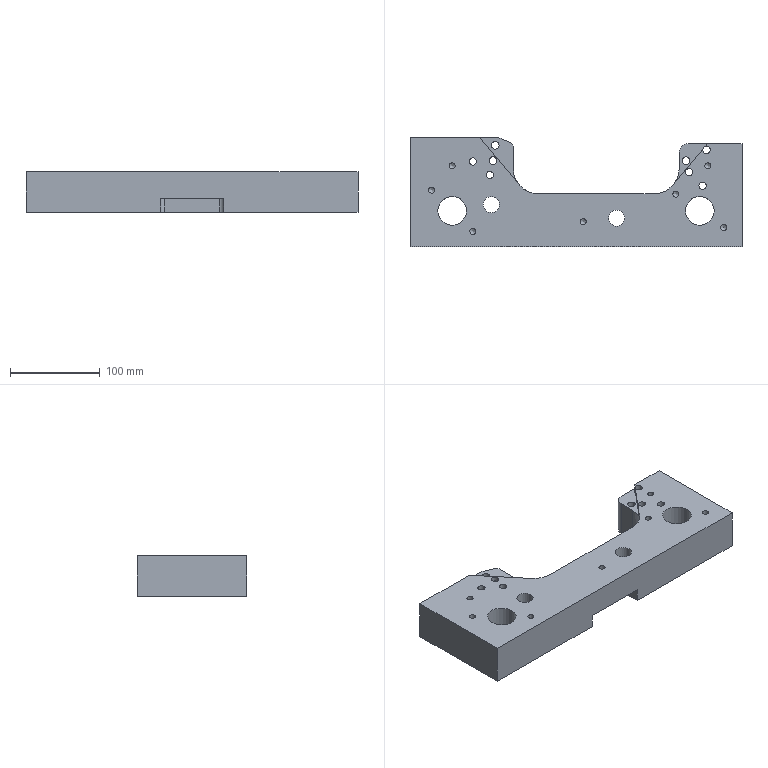Part | STEP file | 302_id2326_x_t | 1 solid | 74 faces | box 370 x 122 x 45 mm | volume 1312955 mm3 | cylinder 35 | plane 22 | cone 17 | commonest cylinder face diameters 6.8 x11 8 x4 8.5 x4 5.2 x2 10 x2 14 x2